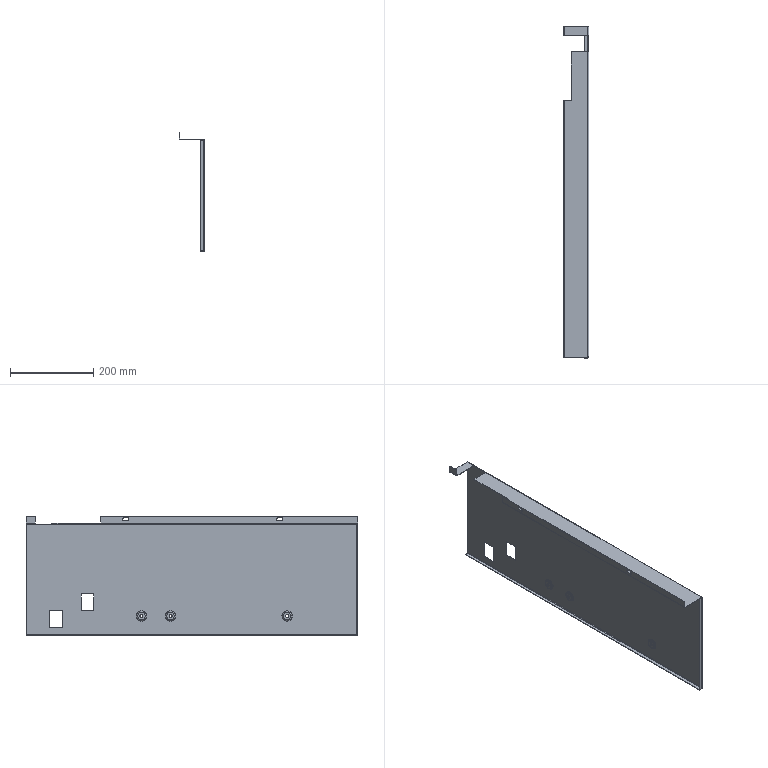Part | STEP file | 1 solid | 124 faces | box 62 x 797 x 286 mm | volume 329072 mm3 | plane 68 | cylinder 32 | torus 24 | commonest cylinder face diameters 7 x10 20 x6 22.4 x6 2 x5 4.4 x5